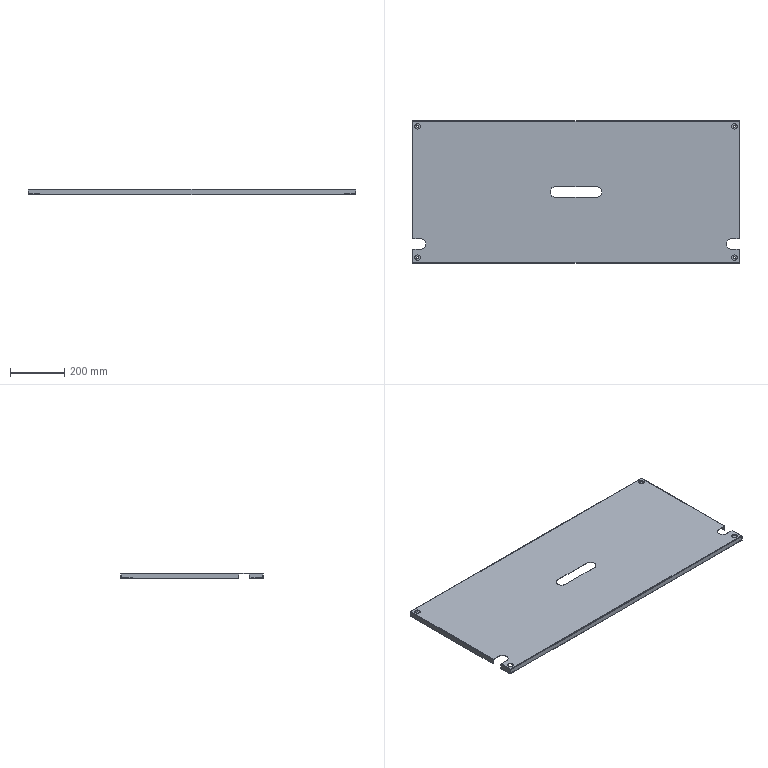Part | STEP file | Box sheet metal 2_default<machined> | 5 solids | 132 faces | box 1203 x 522 x 20 mm | volume 1030115 mm3 | plane 74 | cylinder 38 | spline 20 | commonest cylinder face diameters 7 x8 20 x8 1.5 x6 4.5 x6 40 x6 2 x4